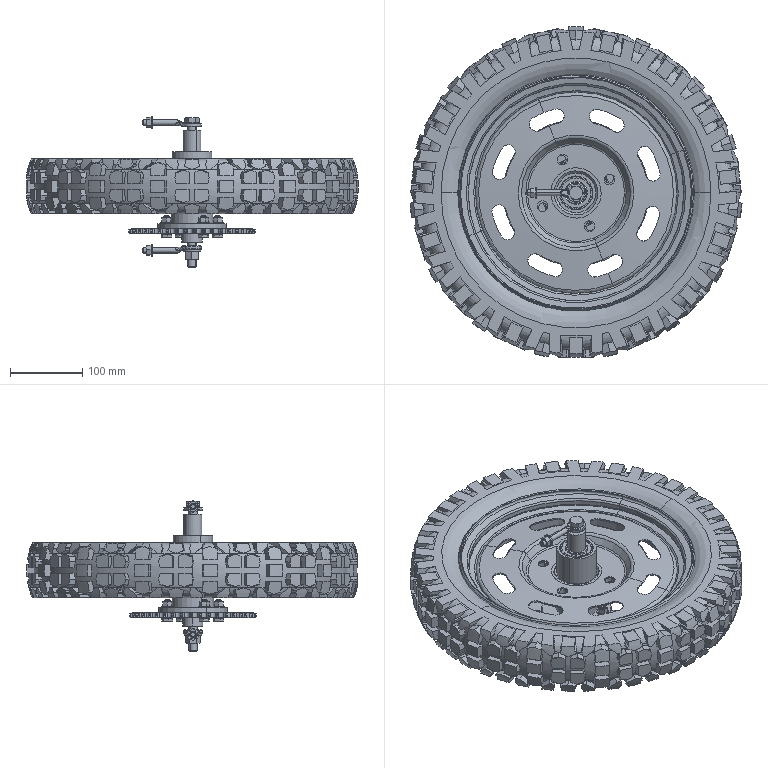Part | SolidWorks | 36 solids | 4166 faces | volume 3150338 mm3 | plane 2772 | cylinder 565 | torus 401 | cone 200 | sphere 192 | spline 36 | commonest cylinder face diameters 12.099 x88 22.269 x88 8.653 x54 176 x43 20 x30 8 x24